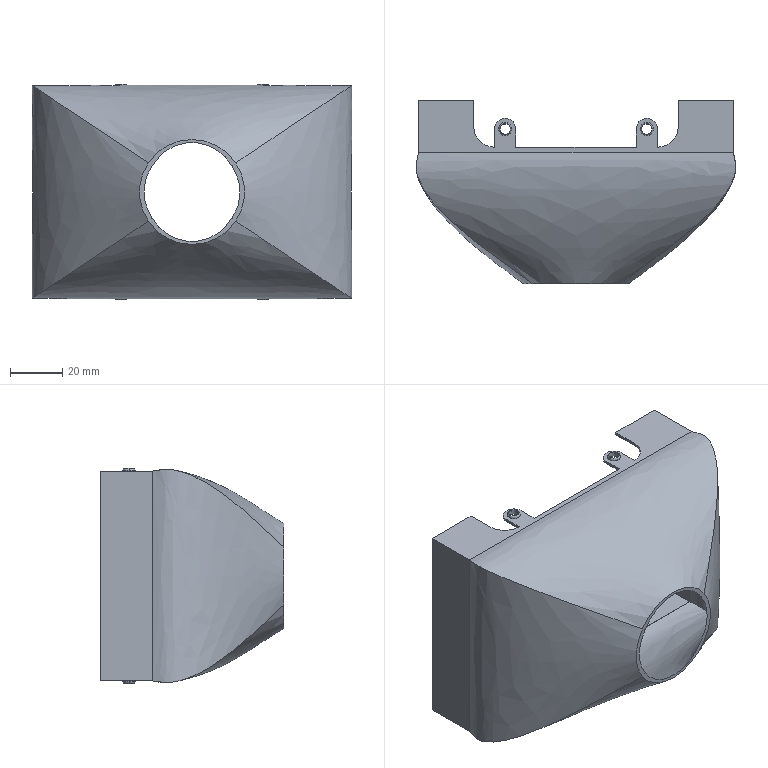Part | SolidWorks | features MirrorPattern 8, ICE 6, Blend 1, Fillet 1, RefAxis 1, Shell 1 | 1 solid | 71 faces | box 121.759 x 70.429 x 82 mm | volume 20309 mm3 | plane 31 | cylinder 24 | torus 8 | spline 8 | commonest cylinder face diameters 4 x8 5 x8 8 x4 16 x4